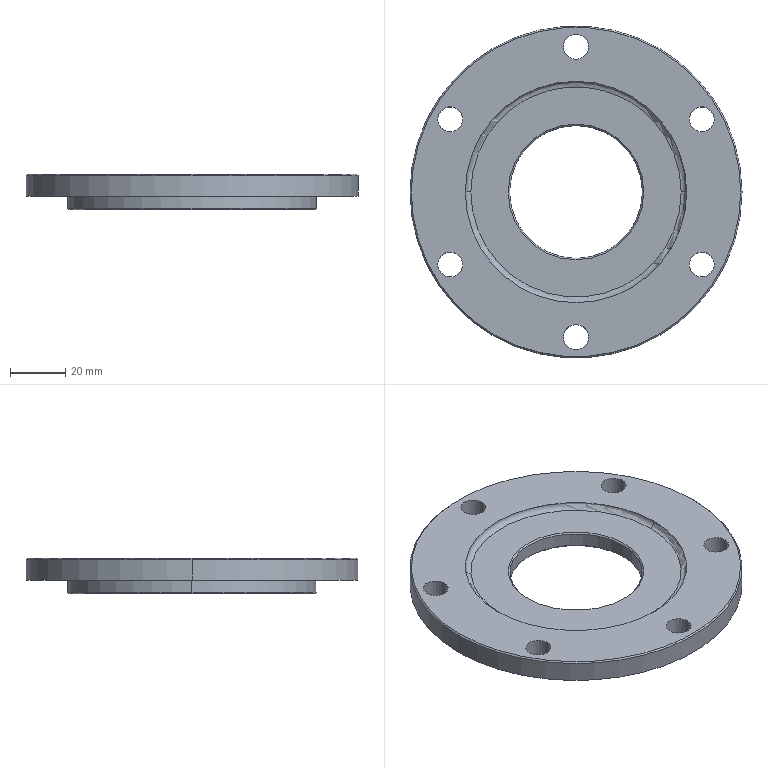Part | SolidWorks | features ICE 3, Chamfer 2, Extrusion 1, Fillet 1 | 1 solid | 35 faces | box 120 x 120 x 13 mm | volume 73283 mm3 | cylinder 20 | cone 8 | plane 5 | torus 2 | commonest cylinder face diameters 9 x12 48 x2 80 x2 90 x2 120 x2
STEP:
#1=CARTESIAN_POINT('',(-24.,0.,5.5));
#2=VERTEX_POINT('',#1);
#3=CARTESIAN_POINT('',(24.,0.,5.5));
#4=VERTEX_POINT('',#3);
#5=CARTESIAN_POINT('',(0.,0.,5.5));
#6=DIRECTION('',(0.,0.,1.));
#7=DIRECTION('',(1.,0.,0.));
#8=AXIS2_PLACEMENT_3D('',#5,#6,#7);
#9=CIRCLE('',#8,24.);
#10=EDGE_CURVE('',#2,#4,#9,.T.);
#11=ORIENTED_EDGE('',*,*,#10,.F.);
#12=CARTESIAN_POINT('',(-24.5,0.,6.));
#13=VERTEX_POINT('',#12);
#14=CARTESIAN_POINT('',(-24.,0.,5.5));
#15=DIRECTION('',(-0.7071,0.,0.7071));
#16=VECTOR('',#15,1000.);
#17=LINE('',#14,#16);
#18=EDGE_CURVE('',#2,#13,#17,.T.);
#19=ORIENTED_EDGE('',*,*,#18,.T.);
#20=CARTESIAN_POINT('',(24.5,0.,6.));
#21=VERTEX_POINT('',#20);
#22=CARTESIAN_POINT('',(0.,0.,6.));
#23=DIRECTION('',(0.,0.,-1.));
#24=DIRECTION('',(1.,0.,0.));
#25=AXIS2_PLACEMENT_3D('',#22,#23,#24);
#26=CIRCLE('',#25,24.5);
#27=EDGE_CURVE('',#21,#13,#26,.T.);
#28=ORIENTED_EDGE('',*,*,#27,.F.);
#29=CARTESIAN_POINT('',(24.,0.,5.5));
#30=DIRECTION('',(0.7071,0.,0.7071));
#31=VECTOR('',#30,1000.);
#32=LINE('',#29,#31);
#33=EDGE_CURVE('',#4,#21,#32,.T.);
#34=ORIENTED_EDGE('',*,*,#33,.F.);
#35=EDGE_LOOP('',(#11,#19,#28,#34));
#36=FACE_OUTER_BOUND('',#35,.T.);
#37=CARTESIAN_POINT('',(0.,0.,5.5));
#38=DIRECTION('',(0.,0.,1.));
#39=DIRECTION('',(1.,0.,0.));
#40=AXIS2_PLACEMENT_3D('',#37,#38,#39);
#41=CONICAL_SURFACE('',#40,24.,0.7854);
#42=ADVANCED_FACE('',(#36),#41,.F.);
#43=CARTESIAN_POINT('',(24.,0.,0.5));
#44=VERTEX_POINT('',#43);
#45=CARTESIAN_POINT('',(-24.,0.,0.5));
#46=VERTEX_POINT('',#45);
#47=CARTESIAN_POINT('',(0.,0.,0.5));
#48=DIRECTION('',(0.,0.,-1.));
#49=DIRECTION('',(1.,0.,0.));
#50=AXIS2_PLACEMENT_3D('',#47,#48,#49);
#51=CIRCLE('',#50,24.);
#52=EDGE_CURVE('',#44,#46,#51,.T.);
#53=ORIENTED_EDGE('',*,*,#52,.F.);
#54=CARTESIAN_POINT('',(24.5,0.,0.));
#55=VERTEX_POINT('',#54);
#56=CARTESIAN_POINT('',(24.5,0.,0.));
#57=DIRECTION('',(0.7071,0.,-0.7071));
#58=VECTOR('',#57,1000.);
#59=LINE('',#56,#58);
#60=EDGE_CURVE('',#44,#55,#59,.T.);
#61=ORIENTED_EDGE('',*,*,#60,.T.);
#62=CARTESIAN_POINT('',(-24.5,0.,0.));
#63=VERTEX_POINT('',#62);
#64=CARTESIAN_POINT('',(0.,0.,0.));
#65=DIRECTION('',(0.,0.,1.));
#66=DIRECTION('',(1.,0.,0.));
#67=AXIS2_PLACEMENT_3D('',#64,#65,#66);
#68=CIRCLE('',#67,24.5);
#69=EDGE_CURVE('',#63,#55,#68,.T.);
#70=ORIENTED_EDGE('',*,*,#69,.F.);
#71=CARTESIAN_POINT('',(-24.5,0.,0.));
#72=DIRECTION('',(-0.7071,0.,-0.7071));
#73=VECTOR('',#72,1000.);
#74=LINE('',#71,#73);
#75=EDGE_CURVE('',#46,#63,#74,.T.);
#76=ORIENTED_EDGE('',*,*,#75,.F.);
#77=EDGE_LOOP('',(#53,#61,#70,#76));
#78=FACE_OUTER_BOUND('',#77,.T.);
#79=CARTESIAN_POINT('',(0.,0.,0.));
#80=DIRECTION('',(0.,0.,-1.));
#81=DIRECTION('',(-1.,0.,0.));
#82=AXIS2_PLACEMENT_3D('',#79,#80,#81);
#83=CONICAL_SURFACE('',#82,24.5,0.7854);
#84=ADVANCED_FACE('',(#78),#83,.F.);
#85=ORIENTED_EDGE('',*,*,#52,.T.);
#86=CARTESIAN_POINT('',(-24.,0.,-4.));
#87=DIRECTION('',(0.,0.,1.));
#88=VECTOR('',#87,1000.);
#89=LINE('',#86,#88);
#90=EDGE_CURVE('',#46,#2,#89,.T.);
#91=ORIENTED_EDGE('',*,*,#90,.T.);
#92=ORIENTED_EDGE('',*,*,#10,.T.);
#93=CARTESIAN_POINT('',(24.,0.,-4.));
#94=DIRECTION('',(0.,0.,1.));
#95=VECTOR('',#94,1000.);
#96=LINE('',#93,#95);
#97=EDGE_CURVE('',#44,#4,#96,.T.);
#98=ORIENTED_EDGE('',*,*,#97,.F.);
#99=EDGE_LOOP('',(#85,#91,#92,#98));
#100=FACE_OUTER_BOUND('',#99,.T.);
#101=CARTESIAN_POINT('',(0.,0.,-4.));
#102=DIRECTION('',(0.,0.,1.));
#103=DIRECTION('',(1.,0.,0.));
#104=AXIS2_PLACEMENT_3D('',#101,#102,#103);
#105=CYLINDRICAL_SURFACE('',#104,24.);
#106=ADVANCED_FACE('',(#100),#105,.F.);
#107=CARTESIAN_POINT('',(-38.,0.,6.));
#108=VERTEX_POINT('',#107);
#109=CARTESIAN_POINT('',(38.,0.,6.));
#110=VERTEX_POINT('',#109);
#111=CARTESIAN_POINT('',(0.,0.,6.));
#112=DIRECTION('',(0.,0.,1.));
#113=DIRECTION('',(1.,0.,0.));
#114=AXIS2_PLACEMENT_3D('',#111,#112,#113);
#115=CIRCLE('',#114,38.);
#116=EDGE_CURVE('',#108,#110,#115,.T.);
#117=ORIENTED_EDGE('',*,*,#116,.F.);
#118=CARTESIAN_POINT('',(-40.,0.,8.));
#119=VERTEX_POINT('',#118);
#120=CARTESIAN_POINT('',(-38.,0.,8.));
#121=DIRECTION('',(0.,1.,0.));
#122=DIRECTION('',(-1.,0.,0.));
#123=AXIS2_PLACEMENT_3D('',#120,#121,#122);
#124=CIRCLE('',#123,2.);
#125=EDGE_CURVE('',#108,#119,#124,.T.);
#126=ORIENTED_EDGE('',*,*,#125,.T.);
#127=CARTESIAN_POINT('',(40.,0.,8.));
#128=VERTEX_POINT('',#127);
#129=CARTESIAN_POINT('',(0.,0.,8.));
#130=DIRECTION('',(0.,0.,1.));
#131=DIRECTION('',(1.,0.,0.));
#132=AXIS2_PLACEMENT_3D('',#129,#130,#131);
#133=CIRCLE('',#132,40.);
#134=EDGE_CURVE('',#119,#128,#133,.T.);
#135=ORIENTED_EDGE('',*,*,#134,.T.);
#136=CARTESIAN_POINT('',(38.,0.,8.));
#137=DIRECTION('',(0.,-1.,0.));
#138=DIRECTION('',(0.,0.,-1.));
#139=AXIS2_PLACEMENT_3D('',#136,#137,#138);
#140=CIRCLE('',#139,2.);
#141=EDGE_CURVE('',#110,#128,#140,.T.);
#142=ORIENTED_EDGE('',*,*,#141,.F.);
#143=EDGE_LOOP('',(#117,#126,#135,#142));
#144=FACE_OUTER_BOUND('',#143,.T.);
#145=CARTESIAN_POINT('',(0.,0.,8.));
#146=DIRECTION('',(0.,0.,1.));
#147=DIRECTION('',(1.,0.,0.));
#148=AXIS2_PLACEMENT_3D('',#145,#146,#147);
#149=TOROIDAL_SURFACE('',#148,38.,2.);
#150=ADVANCED_FACE('',(#144),#149,.F.);
#151=CARTESIAN_POINT('',(59.5,0.,8.));
#152=VERTEX_POINT('',#151);
#153=CARTESIAN_POINT('',(-59.5,0.,8.));
#154=VERTEX_POINT('',#153);
#155=CARTESIAN_POINT('',(0.,0.,8.));
#156=DIRECTION('',(0.,0.,1.));
#157=DIRECTION('',(1.,0.,0.));
#158=AXIS2_PLACEMENT_3D('',#155,#156,#157);
#159=CIRCLE('',#158,59.5);
#160=EDGE_CURVE('',#152,#154,#159,.T.);
#161=ORIENTED_EDGE('',*,*,#160,.F.);
#162=CARTESIAN_POINT('',(60.,0.,7.5));
#163=VERTEX_POINT('',#162);
#164=CARTESIAN_POINT('',(59.5,0.,8.));
#165=DIRECTION('',(0.7071,0.,-0.7071));
#166=VECTOR('',#165,1000.);
#167=LINE('',#164,#166);
#168=EDGE_CURVE('',#152,#163,#167,.T.);
#169=ORIENTED_EDGE('',*,*,#168,.T.);
#170=CARTESIAN_POINT('',(-60.,0.,7.5));
#171=VERTEX_POINT('',#170);
#172=CARTESIAN_POINT('',(0.,0.,7.5));
#173=DIRECTION('',(0.,0.,-1.));
#174=DIRECTION('',(1.,0.,0.));
#175=AXIS2_PLACEMENT_3D('',#172,#173,#174);
#176=CIRCLE('',#175,60.);
#177=EDGE_CURVE('',#171,#163,#176,.T.);
#178=ORIENTED_EDGE('',*,*,#177,.F.);
#179=CARTESIAN_POINT('',(-59.5,0.,8.));
#180=DIRECTION('',(-0.7071,0.,-0.7071));
#181=VECTOR('',#180,1000.);
#182=LINE('',#179,#181);
#183=EDGE_CURVE('',#154,#171,#182,.T.);
#184=ORIENTED_EDGE('',*,*,#183,.F.);
#185=EDGE_LOOP('',(#161,#169,#178,#184));
#186=FACE_OUTER_BOUND('',#185,.T.);
#187=CARTESIAN_POINT('',(0.,0.,8.));
#188=DIRECTION('',(0.,0.,-1.));
#189=DIRECTION('',(-1.,0.,0.));
#190=AXIS2_PLACEMENT_3D('',#187,#188,#189);
#191=CONICAL_SURFACE('',#190,59.5,0.7854);
#192=ADVANCED_FACE('',(#186),#191,.T.);
#193=CARTESIAN_POINT('',(-44.5,0.,-5.));
#194=VERTEX_POINT('',#193);
#195=CARTESIAN_POINT('',(44.5,0.,-5.));
#196=VERTEX_POINT('',#195);
#197=CARTESIAN_POINT('',(0.,0.,-5.));
#198=DIRECTION('',(0.,0.,-1.));
#199=DIRECTION('',(-1.,0.,0.));
#200=AXIS2_PLACEMENT_3D('',#197,#198,#199);
#201=CIRCLE('',#200,44.5);
#202=EDGE_CURVE('',#194,#196,#201,.T.);
#203=ORIENTED_EDGE('',*,*,#202,.F.);
#204=CARTESIAN_POINT('',(-45.,0.,-4.5));
#205=VERTEX_POINT('',#204);
#206=CARTESIAN_POINT('',(-44.5,0.,-5.));
#207=DIRECTION('',(-0.7071,0.,0.7071));
#208=VECTOR('',#207,1000.);
#209=LINE('',#206,#208);
#210=EDGE_CURVE('',#194,#205,#209,.T.);
#211=ORIENTED_EDGE('',*,*,#210,.T.);
#212=CARTESIAN_POINT('',(45.,0.,-4.5));
#213=VERTEX_POINT('',#212);
#214=CARTESIAN_POINT('',(0.,0.,-4.5));
#215=DIRECTION('',(0.,0.,1.));
#216=DIRECTION('',(-1.,0.,0.));
#217=AXIS2_PLACEMENT_3D('',#214,#215,#216);
#218=CIRCLE('',#217,45.);
#219=EDGE_CURVE('',#213,#205,#218,.T.);
#220=ORIENTED_EDGE('',*,*,#219,.F.);
#221=CARTESIAN_POINT('',(44.5,0.,-5.));
#222=DIRECTION('',(0.7071,0.,0.7071));
#223=VECTOR('',#222,1000.);
#224=LINE('',#221,#223);
#225=EDGE_CURVE('',#196,#213,#224,.T.);
#226=ORIENTED_EDGE('',*,*,#225,.F.);
#227=EDGE_LOOP('',(#203,#211,#220,#226));
#228=FACE_OUTER_BOUND('',#227,.T.);
#229=CARTESIAN_POINT('',(0.,0.,-5.));
#230=DIRECTION('',(0.,0.,1.));
#231=DIRECTION('',(1.,0.,0.));
#232=AXIS2_PLACEMENT_3D('',#229,#230,#231);
#233=CONICAL_SURFACE('',#232,44.5,0.7854);
#234=ADVANCED_FACE('',(#228),#233,.T.);
#235=CARTESIAN_POINT('',(40.,0.,-5.));
#236=VERTEX_POINT('',#235);
#237=CARTESIAN_POINT('',(-40.,0.,-5.));
#238=VERTEX_POINT('',#237);
#239=CARTESIAN_POINT('',(0.,0.,-5.));
#240=DIRECTION('',(0.,0.,-1.));
#241=DIRECTION('',(-1.,0.,0.));
#242=AXIS2_PLACEMENT_3D('',#239,#240,#241);
#243=CIRCLE('',#242,40.);
#244=EDGE_CURVE('',#236,#238,#243,.T.);
#245=ORIENTED_EDGE('',*,*,#244,.T.);
#246=CARTESIAN_POINT('',(-40.,0.,0.));
#247=VERTEX_POINT('',#246);
#248=CARTESIAN_POINT('',(-40.,0.,-5.));
#249=DIRECTION('',(0.,0.,1.));
#250=VECTOR('',#249,1000.);
#251=LINE('',#248,#250);
#252=EDGE_CURVE('',#238,#247,#251,.T.);
#253=ORIENTED_EDGE('',*,*,#252,.T.);
#254=CARTESIAN_POINT('',(40.,0.,0.));
#255=VERTEX_POINT('',#254);
#256=CARTESIAN_POINT('',(0.,0.,0.));
#257=DIRECTION('',(0.,0.,-1.));
#258=DIRECTION('',(-1.,0.,0.));
#259=AXIS2_PLACEMENT_3D('',#256,#257,#258);
#260=CIRCLE('',#259,40.);
#261=EDGE_CURVE('',#255,#247,#260,.T.);
#262=ORIENTED_EDGE('',*,*,#261,.F.);
#263=CARTESIAN_POINT('',(40.,0.,-5.));
#264=DIRECTION('',(0.,0.,1.));
#265=VECTOR('',#264,1000.);
#266=LINE('',#263,#265);
#267=EDGE_CURVE('',#236,#255,#266,.T.);
#268=ORIENTED_EDGE('',*,*,#267,.F.);
#269=EDGE_LOOP('',(#245,#253,#262,#268));
#270=FACE_OUTER_BOUND('',#269,.T.);
#271=CARTESIAN_POINT('',(0.,0.,-5.));
#272=DIRECTION('',(0.,0.,1.));
#273=DIRECTION('',(1.,0.,0.));
#274=AXIS2_PLACEMENT_3D('',#271,#272,#273);
#275=CYLINDRICAL_SURFACE('',#274,40.);
#276=ADVANCED_FACE('',(#270),#275,.F.);
#277=ORIENTED_EDGE('',*,*,#219,.T.);
#278=CARTESIAN_POINT('',(-45.,0.,0.));
#279=VERTEX_POINT('',#278);
#280=CARTESIAN_POINT('',(-45.,0.,-5.));
#281=DIRECTION('',(0.,0.,1.));
#282=VECTOR('',#281,1000.);
#283=LINE('',#280,#282);
#284=EDGE_CURVE('',#205,#279,#283,.T.);
#285=ORIENTED_EDGE('',*,*,#284,.T.);
#286=CARTESIAN_POINT('',(45.,0.,0.));
#287=VERTEX_POINT('',#286);
#288=CARTESIAN_POINT('',(0.,0.,0.));
#289=DIRECTION('',(0.,0.,-1.));
#290=DIRECTION('',(1.,0.,0.));
#291=AXIS2_PLACEMENT_3D('',#288,#289,#290);
#292=CIRCLE('',#291,45.);
#293=EDGE_CURVE('',#279,#287,#292,.T.);
#294=ORIENTED_EDGE('',*,*,#293,.T.);
#295=CARTESIAN_POINT('',(45.,0.,-5.));
#296=DIRECTION('',(0.,0.,1.));
#297=VECTOR('',#296,1000.);
#298=LINE('',#295,#297);
#299=EDGE_CURVE('',#213,#287,#298,.T.);
#300=ORIENTED_EDGE('',*,*,#299,.F.);
#301=EDGE_LOOP('',(#277,#285,#294,#300));
#302=FACE_OUTER_BOUND('',#301,.T.);
#303=CARTESIAN_POINT('',(0.,0.,-5.));
#304=DIRECTION('',(0.,0.,1.));
#305=DIRECTION('',(1.,0.,0.));
#306=AXIS2_PLACEMENT_3D('',#303,#304,#305);
#307=CYLINDRICAL_SURFACE('',#306,45.);
#308=ADVANCED_FACE('',(#302),#307,.T.);
#309=CARTESIAN_POINT('',(-49.966,26.25,8.));
#310=VERTEX_POINT('',#309);
#311=CARTESIAN_POINT('',(-40.966,26.25,8.));
#312=VERTEX_POINT('',#311);
#313=CARTESIAN_POINT('',(-45.466,26.25,8.));
#314=DIRECTION('',(0.,0.,1.));
#315=DIRECTION('',(1.,0.,0.));
#316=AXIS2_PLACEMENT_3D('',#313,#314,#315);
#317=CIRCLE('',#316,4.5);
#318=EDGE_CURVE('',#310,#312,#317,.T.);
#319=ORIENTED_EDGE('',*,*,#318,.T.);
#320=CARTESIAN_POINT('',(-40.966,26.25,0.));
#321=VERTEX_POINT('',#320);
#322=CARTESIAN_POINT('',(-40.966,26.25,8.));
#323=DIRECTION('',(0.,0.,-1.));
#324=VECTOR('',#323,1000.);
#325=LINE('',#322,#324);
#326=EDGE_CURVE('',#312,#321,#325,.T.);
#327=ORIENTED_EDGE('',*,*,#326,.T.);
#328=CARTESIAN_POINT('',(-49.966,26.25,0.));
#329=VERTEX_POINT('',#328);
#330=CARTESIAN_POINT('',(-45.466,26.25,0.));
#331=DIRECTION('',(0.,0.,1.));
#332=DIRECTION('',(1.,0.,0.));
#333=AXIS2_PLACEMENT_3D('',#330,#331,#332);
#334=CIRCLE('',#333,4.5);
#335=EDGE_CURVE('',#329,#321,#334,.T.);
#336=ORIENTED_EDGE('',*,*,#335,.F.);
#337=CARTESIAN_POINT('',(-49.966,26.25,8.));
#338=DIRECTION('',(0.,0.,-1.));
#339=VECTOR('',#338,1000.);
#340=LINE('',#337,#339);
#341=EDGE_CURVE('',#310,#329,#340,.T.);
#342=ORIENTED_EDGE('',*,*,#341,.F.);
#343=EDGE_LOOP('',(#319,#327,#336,#342));
#344=FACE_OUTER_BOUND('',#343,.T.);
#345=CARTESIAN_POINT('',(-45.466,26.25,8.));
#346=DIRECTION('',(0.,0.,-1.));
#347=DIRECTION('',(-1.,0.,0.));
#348=AXIS2_PLACEMENT_3D('',#345,#346,#347);
#349=CYLINDRICAL_SURFACE('',#348,4.5);
#350=ADVANCED_FACE('',(#344),#349,.F.);
#351=CARTESIAN_POINT('',(-49.966,-26.25,8.));
#352=VERTEX_POINT('',#351);
#353=CARTESIAN_POINT('',(-40.966,-26.25,8.));
#354=VERTEX_POINT('',#353);
#355=CARTESIAN_POINT('',(-45.466,-26.25,8.));
#356=DIRECTION('',(0.,0.,1.));
#357=DIRECTION('',(1.,0.,0.));
#358=AXIS2_PLACEMENT_3D('',#355,#356,#357);
#359=CIRCLE('',#358,4.5);
#360=EDGE_CURVE('',#352,#354,#359,.T.);
#361=ORIENTED_EDGE('',*,*,#360,.T.);
#362=CARTESIAN_POINT('',(-40.966,-26.25,0.));
#363=VERTEX_POINT('',#362);
#364=CARTESIAN_POINT('',(-40.966,-26.25,8.));
#365=DIRECTION('',(0.,0.,-1.));
#366=VECTOR('',#365,1000.);
#367=LINE('',#364,#366);
#368=EDGE_CURVE('',#354,#363,#367,.T.);
#369=ORIENTED_EDGE('',*,*,#368,.T.);
#370=CARTESIAN_POINT('',(-49.966,-26.25,0.));
#371=VERTEX_POINT('',#370);
#372=CARTESIAN_POINT('',(-45.466,-26.25,0.));
#373=DIRECTION('',(0.,0.,1.));
#374=DIRECTION('',(1.,0.,0.));
#375=AXIS2_PLACEMENT_3D('',#372,#373,#374);
#376=CIRCLE('',#375,4.5);
#377=EDGE_CURVE('',#371,#363,#376,.T.);
#378=ORIENTED_EDGE('',*,*,#377,.F.);
#379=CARTESIAN_POINT('',(-49.966,-26.25,8.));
#380=DIRECTION('',(0.,0.,-1.));
#381=VECTOR('',#380,1000.);
#382=LINE('',#379,#381);
#383=EDGE_CURVE('',#352,#371,#382,.T.);
#384=ORIENTED_EDGE('',*,*,#383,.F.);
#385=EDGE_LOOP('',(#361,#369,#378,#384));
#386=FACE_OUTER_BOUND('',#385,.T.);
#387=CARTESIAN_POINT('',(-45.466,-26.25,8.));
#388=DIRECTION('',(0.,0.,-1.));
#389=DIRECTION('',(-1.,0.,0.));
#390=AXIS2_PLACEMENT_3D('',#387,#388,#389);
#391=CYLINDRICAL_SURFACE('',#390,4.5);
#392=ADVANCED_FACE('',(#386),#391,.F.);
#393=CARTESIAN_POINT('',(-4.5,-52.5,8.));
#394=VERTEX_POINT('',#393);
#395=CARTESIAN_POINT('',(4.5,-52.5,8.));
#396=VERTEX_POINT('',#395);
#397=CARTESIAN_POINT('',(0.,-52.5,8.));
#398=DIRECTION('',(0.,0.,1.));
#399=DIRECTION('',(1.,0.,0.));
#400=AXIS2_PLACEMENT_3D('',#397,#398,#399);
#401=CIRCLE('',#400,4.5);
#402=EDGE_CURVE('',#394,#396,#401,.T.);
#403=ORIENTED_EDGE('',*,*,#402,.T.);
#404=CARTESIAN_POINT('',(4.5,-52.5,0.));
#405=VERTEX_POINT('',#404);
#406=CARTESIAN_POINT('',(4.5,-52.5,8.));
#407=DIRECTION('',(0.,0.,-1.));
#408=VECTOR('',#407,1000.);
#409=LINE('',#406,#408);
#410=EDGE_CURVE('',#396,#405,#409,.T.);
#411=ORIENTED_EDGE('',*,*,#410,.T.);
#412=CARTESIAN_POINT('',(-4.5,-52.5,0.));
#413=VERTEX_POINT('',#412);
#414=CARTESIAN_POINT('',(0.,-52.5,0.));
#415=DIRECTION('',(0.,0.,1.));
#416=DIRECTION('',(1.,0.,0.));
#417=AXIS2_PLACEMENT_3D('',#414,#415,#416);
#418=CIRCLE('',#417,4.5);
#419=EDGE_CURVE('',#413,#405,#418,.T.);
#420=ORIENTED_EDGE('',*,*,#419,.F.);
#421=CARTESIAN_POINT('',(-4.5,-52.5,8.));
#422=DIRECTION('',(0.,0.,-1.));
#423=VECTOR('',#422,1000.);
#424=LINE('',#421,#423);
#425=EDGE_CURVE('',#394,#413,#424,.T.);
#426=ORIENTED_EDGE('',*,*,#425,.F.);
#427=EDGE_LOOP('',(#403,#411,#420,#426));
#428=FACE_OUTER_BOUND('',#427,.T.);
#429=CARTESIAN_POINT('',(0.,-52.5,8.));
#430=DIRECTION('',(0.,0.,-1.));
#431=DIRECTION('',(-1.,0.,0.));
#432=AXIS2_PLACEMENT_3D('',#429,#430,#431);
#433=CYLINDRICAL_SURFACE('',#432,4.5);
#434=ADVANCED_FACE('',(#428),#433,.F.);
#435=CARTESIAN_POINT('',(40.966,-26.25,8.));
#436=VERTEX_POINT('',#435);
#437=CARTESIAN_POINT('',(49.966,-26.25,8.));
#438=VERTEX_POINT('',#437);
#439=CARTESIAN_POINT('',(45.466,-26.25,8.));
#440=DIRECTION('',(0.,0.,1.));
#441=DIRECTION('',(1.,0.,0.));
#442=AXIS2_PLACEMENT_3D('',#439,#440,#441);
#443=CIRCLE('',#442,4.5);
#444=EDGE_CURVE('',#436,#438,#443,.T.);
#445=ORIENTED_EDGE('',*,*,#444,.T.);
#446=CARTESIAN_POINT('',(49.966,-26.25,0.));
#447=VERTEX_POINT('',#446);
#448=CARTESIAN_POINT('',(49.966,-26.25,8.));
#449=DIRECTION('',(0.,0.,-1.));
#450=VECTOR('',#449,1000.);
#451=LINE('',#448,#450);
#452=EDGE_CURVE('',#438,#447,#451,.T.);
#453=ORIENTED_EDGE('',*,*,#452,.T.);
#454=CARTESIAN_POINT('',(40.966,-26.25,0.));
#455=VERTEX_POINT('',#454);
#456=CARTESIAN_POINT('',(45.466,-26.25,0.));
#457=DIRECTION('',(0.,0.,1.));
#458=DIRECTION('',(1.,0.,0.));
#459=AXIS2_PLACEMENT_3D('',#456,#457,#458);
#460=CIRCLE('',#459,4.5);
#461=EDGE_CURVE('',#455,#447,#460,.T.);
#462=ORIENTED_EDGE('',*,*,#461,.F.);
#463=CARTESIAN_POINT('',(40.966,-26.25,8.));
#464=DIRECTION('',(0.,0.,-1.));
#465=VECTOR('',#464,1000.);
#466=LINE('',#463,#465);
#467=EDGE_CURVE('',#436,#455,#466,.T.);
#468=ORIENTED_EDGE('',*,*,#467,.F.);
#469=EDGE_LOOP('',(#445,#453,#462,#468));
#470=FACE_OUTER_BOUND('',#469,.T.);
#471=CARTESIAN_POINT('',(45.466,-26.25,8.));
#472=DIRECTION('',(0.,0.,-1.));
#473=DIRECTION('',(-1.,0.,0.));
#474=AXIS2_PLACEMENT_3D('',#471,#472,#473);
#475=CYLINDRICAL_SURFACE('',#474,4.5);
#476=ADVANCED_FACE('',(#470),#475,.F.);
#477=CARTESIAN_POINT('',(40.966,26.25,8.));
#478=VERTEX_POINT('',#477);
#479=CARTESIAN_POINT('',(49.966,26.25,8.));
#480=VERTEX_POINT('',#479);
#481=CARTESIAN_POINT('',(45.466,26.25,8.));
#482=DIRECTION('',(0.,0.,1.));
#483=DIRECTION('',(1.,0.,0.));
#484=AXIS2_PLACEMENT_3D('',#481,#482,#483);
#485=CIRCLE('',#484,4.5);
#486=EDGE_CURVE('',#478,#480,#485,.T.);
#487=ORIENTED_EDGE('',*,*,#486,.T.);
#488=CARTESIAN_POINT('',(49.966,26.25,0.));
#489=VERTEX_POINT('',#488);
#490=CARTESIAN_POINT('',(49.966,26.25,8.));
#491=DIRECTION('',(0.,0.,-1.));
#492=VECTOR('',#491,1000.);
#493=LINE('',#490,#492);
#494=EDGE_CURVE('',#480,#489,#493,.T.);
#495=ORIENTED_EDGE('',*,*,#494,.T.);
#496=CARTESIAN_POINT('',(40.966,26.25,0.));
#497=VERTEX_POINT('',#496);
#498=CARTESIAN_POINT('',(45.466,26.25,0.));
#499=DIRECTION('',(0.,0.,1.));
#500=DIRECTION('',(1.,0.,0.));
#501=AXIS2_PLACEMENT_3D('',#498,#499,#500);
#502=CIRCLE('',#501,4.5);
#503=EDGE_CURVE('',#497,#489,#502,.T.);
#504=ORIENTED_EDGE('',*,*,#503,.F.);
#505=CARTESIAN_POINT('',(40.966,26.25,8.));
#506=DIRECTION('',(0.,0.,-1.));
#507=VECTOR('',#506,1000.);
#508=LINE('',#505,#507);
#509=EDGE_CURVE('',#478,#497,#508,.T.);
#510=ORIENTED_EDGE('',*,*,#509,.F.);
#511=EDGE_LOOP('',(#487,#495,#504,#510));
#512=FACE_OUTER_BOUND('',#511,.T.);
#513=CARTESIAN_POINT('',(45.466,26.25,8.));
#514=DIRECTION('',(0.,0.,-1.));
#515=DIRECTION('',(-1.,0.,0.));
#516=AXIS2_PLACEMENT_3D('',#513,#514,#515);
#517=CYLINDRICAL_SURFACE('',#516,4.5);
#518=ADVANCED_FACE('',(#512),#517,.F.);
#519=CARTESIAN_POINT('',(-4.5,52.5,8.));
#520=VERTEX_POINT('',#519);
#521=CARTESIAN_POINT('',(4.5,52.5,8.));
#522=VERTEX_POINT('',#521);
#523=CARTESIAN_POINT('',(0.,52.5,8.));
#524=DIRECTION('',(0.,0.,1.));
#525=DIRECTION('',(1.,0.,0.));
#526=AXIS2_PLACEMENT_3D('',#523,#524,#525);
#527=CIRCLE('',#526,4.5);
#528=EDGE_CURVE('',#520,#522,#527,.T.);
#529=ORIENTED_EDGE('',*,*,#528,.T.);
#530=CARTESIAN_POINT('',(4.5,52.5,0.));
#531=VERTEX_POINT('',#530);
#532=CARTESIAN_POINT('',(4.5,52.5,8.));
#533=DIRECTION('',(0.,0.,-1.));
#534=VECTOR('',#533,1000.);
#535=LINE('',#532,#534);
#536=EDGE_CURVE('',#522,#531,#535,.T.);
#537=ORIENTED_EDGE('',*,*,#536,.T.);
#538=CARTESIAN_POINT('',(-4.5,52.5,0.));
#539=VERTEX_POINT('',#538);
#540=CARTESIAN_POINT('',(0.,52.5,0.));
#541=DIRECTION('',(0.,0.,1.));
#542=DIRECTION('',(1.,0.,0.));
#543=AXIS2_PLACEMENT_3D('',#540,#541,#542);
#544=CIRCLE('',#543,4.5);
#545=EDGE_CURVE('',#539,#531,#544,.T.);
#546=ORIENTED_EDGE('',*,*,#545,.F.);
#547=CARTESIAN_POINT('',(-4.5,52.5,8.));
#548=DIRECTION('',(0.,0.,-1.));
#549=VECTOR('',#548,1000.);
#550=LINE('',#547,#549);
#551=EDGE_CURVE('',#520,#539,#550,.T.);
#552=ORIENTED_EDGE('',*,*,#551,.F.);
#553=EDGE_LOOP('',(#529,#537,#546,#552));
#554=FACE_OUTER_BOUND('',#553,.T.);
#555=CARTESIAN_POINT('',(0.,52.5,8.));
#556=DIRECTION('',(0.,0.,-1.));
#557=DIRECTION('',(-1.,0.,0.));
#558=AXIS2_PLACEMENT_3D('',#555,#556,#557);
#559=CYLINDRICAL_SURFACE('',#558,4.5);
#560=ADVANCED_FACE('',(#554),#559,.F.);
#561=ORIENTED_EDGE('',*,*,#177,.T.);
#562=CARTESIAN_POINT('',(60.,0.,0.));
#563=VERTEX_POINT('',#562);
#564=CARTESIAN_POINT('',(60.,0.,8.));
#565=DIRECTION('',(0.,0.,-1.));
#566=VECTOR('',#565,1000.);
#567=LINE('',#564,#566);
#568=EDGE_CURVE('',#163,#563,#567,.T.);
#569=ORIENTED_EDGE('',*,*,#568,.T.);
#570=CARTESIAN_POINT('',(-60.,0.,0.));
#571=VERTEX_POINT('',#570);
#572=CARTESIAN_POINT('',(0.,0.,0.));
#573=DIRECTION('',(0.,0.,1.));
#574=DIRECTION('',(1.,0.,0.));
#575=AXIS2_PLACEMENT_3D('',#572,#573,#574);
#576=CIRCLE('',#575,60.);
#577=EDGE_CURVE('',#563,#571,#576,.T.);
#578=ORIENTED_EDGE('',*,*,#577,.T.);
#579=CARTESIAN_POINT('',(-60.,0.,8.));
#580=DIRECTION('',(0.,0.,-1.));
#581=VECTOR('',#580,1000.);
#582=LINE('',#579,#581);
#583=EDGE_CURVE('',#171,#571,#582,.T.);
#584=ORIENTED_EDGE('',*,*,#583,.F.);
#585=EDGE_LOOP('',(#561,#569,#578,#584));
#586=FACE_OUTER_BOUND('',#585,.T.);
#587=CARTESIAN_POINT('',(0.,0.,8.));
#588=DIRECTION('',(0.,0.,-1.));
#589=DIRECTION('',(-1.,0.,0.));
#590=AXIS2_PLACEMENT_3D('',#587,#588,#589);
#591=CYLINDRICAL_SURFACE('',#590,60.);
#592=ADVANCED_FACE('',(#586),#591,.T.);
#593=CARTESIAN_POINT('',(0.,0.,8.));
#594=DIRECTION('',(0.,0.,1.));
#595=DIRECTION('',(1.,0.,0.));
#596=AXIS2_PLACEMENT_3D('',#593,#594,#595);
#597=CIRCLE('',#596,40.);
#598=EDGE_CURVE('',#128,#119,#597,.T.);
#599=ORIENTED_EDGE('',*,*,#598,.F.);
#600=ORIENTED_EDGE('',*,*,#134,.F.);
#601=EDGE_LOOP('',(#599,#600));
#602=FACE_BOUND('',#601,.T.);
#603=CARTESIAN_POINT('',(0.,0.,8.));
#604=DIRECTION('',(0.,0.,1.));
#605=DIRECTION('',(1.,0.,0.));
#606=AXIS2_PLACEMENT_3D('',#603,#604,#605);
#607=CIRCLE('',#606,59.5);
#608=EDGE_CURVE('',#154,#152,#607,.T.);
#609=ORIENTED_EDGE('',*,*,#608,.T.);
#610=ORIENTED_EDGE('',*,*,#160,.T.);
#611=EDGE_LOOP('',(#609,#610));
#612=FACE_OUTER_BOUND('',#611,.T.);
#613=ORIENTED_EDGE('',*,*,#360,.F.);
#614=CARTESIAN_POINT('',(-45.466,-26.25,8.));
#615=DIRECTION('',(0.,0.,1.));
#616=DIRECTION('',(1.,0.,0.));
#617=AXIS2_PLACEMENT_3D('',#614,#615,#616);
#618=CIRCLE('',#617,4.5);
#619=EDGE_CURVE('',#354,#352,#618,.T.);
#620=ORIENTED_EDGE('',*,*,#619,.F.);
#621=EDGE_LOOP('',(#613,#620));
#622=FACE_BOUND('',#621,.T.);
#623=ORIENTED_EDGE('',*,*,#444,.F.);
#624=CARTESIAN_POINT('',(45.466,-26.25,8.));
#625=DIRECTION('',(0.,0.,1.));
#626=DIRECTION('',(1.,0.,0.));
#627=AXIS2_PLACEMENT_3D('',#624,#625,#626);
#628=CIRCLE('',#627,4.5);
#629=EDGE_CURVE('',#438,#436,#628,.T.);
#630=ORIENTED_EDGE('',*,*,#629,.F.);
#631=EDGE_LOOP('',(#623,#630));
#632=FACE_BOUND('',#631,.T.);
#633=ORIENTED_EDGE('',*,*,#528,.F.);
#634=CARTESIAN_POINT('',(0.,52.5,8.));
#635=DIRECTION('',(0.,0.,1.));
#636=DIRECTION('',(1.,0.,0.));
#637=AXIS2_PLACEMENT_3D('',#634,#635,#636);
#638=CIRCLE('',#637,4.5);
#639=EDGE_CURVE('',#522,#520,#638,.T.);
#640=ORIENTED_EDGE('',*,*,#639,.F.);
#641=EDGE_LOOP('',(#633,#640));
#642=FACE_BOUND('',#641,.T.);
#643=ORIENTED_EDGE('',*,*,#486,.F.);
#644=CARTESIAN_POINT('',(45.466,26.25,8.));
#645=DIRECTION('',(0.,0.,1.));
#646=DIRECTION('',(1.,0.,0.));
#647=AXIS2_PLACEMENT_3D('',#644,#645,#646);
#648=CIRCLE('',#647,4.5);
#649=EDGE_CURVE('',#480,#478,#648,.T.);
#650=ORIENTED_EDGE('',*,*,#649,.F.);
#651=EDGE_LOOP('',(#643,#650));
#652=FACE_BOUND('',#651,.T.);
#653=ORIENTED_EDGE('',*,*,#402,.F.);
#654=CARTESIAN_POINT('',(0.,-52.5,8.));
#655=DIRECTION('',(0.,0.,1.));
#656=DIRECTION('',(1.,0.,0.));
#657=AXIS2_PLACEMENT_3D('',#654,#655,#656);
#658=CIRCLE('',#657,4.5);
#659=EDGE_CURVE('',#396,#394,#658,.T.);
#660=ORIENTED_EDGE('',*,*,#659,.F.);
#661=EDGE_LOOP('',(#653,#660));
#662=FACE_BOUND('',#661,.T.);
#663=ORIENTED_EDGE('',*,*,#318,.F.);
#664=CARTESIAN_POINT('',(-45.466,26.25,8.));
#665=DIRECTION('',(0.,0.,1.));
#666=DIRECTION('',(1.,0.,0.));
#667=AXIS2_PLACEMENT_3D('',#664,#665,#666);
#668=CIRCLE('',#667,4.5);
#669=EDGE_CURVE('',#312,#310,#668,.T.);
#670=ORIENTED_EDGE('',*,*,#669,.F.);
#671=EDGE_LOOP('',(#663,#670));
#672=FACE_BOUND('',#671,.T.);
#673=CARTESIAN_POINT('',(0.,0.,8.));
#674=DIRECTION('',(0.,0.,1.));
#675=DIRECTION('',(1.,0.,0.));
#676=AXIS2_PLACEMENT_3D('',#673,#674,#675);
#677=PLANE('',#676);
#678=ADVANCED_FACE('',(#602,#612,#622,#632,#642,#652,#662,#672),#677,.T.);
#679=CARTESIAN_POINT('',(0.,0.,0.));
#680=DIRECTION('',(0.,0.,-1.));
#681=DIRECTION('',(1.,0.,0.));
#682=AXIS2_PLACEMENT_3D('',#679,#680,#681);
#683=CIRCLE('',#682,45.);
#684=EDGE_CURVE('',#287,#279,#683,.T.);
#685=ORIENTED_EDGE('',*,*,#684,.F.);
#686=ORIENTED_EDGE('',*,*,#293,.F.);
#687=EDGE_LOOP('',(#685,#686));
#688=FACE_BOUND('',#687,.T.);
#689=CARTESIAN_POINT('',(0.,0.,0.));
#690=DIRECTION('',(0.,0.,1.));
#691=DIRECTION('',(1.,0.,0.));
#692=AXIS2_PLACEMENT_3D('',#689,#690,#691);
#693=CIRCLE('',#692,60.);
#694=EDGE_CURVE('',#571,#563,#693,.T.);
#695=ORIENTED_EDGE('',*,*,#694,.F.);
#696=ORIENTED_EDGE('',*,*,#577,.F.);
#697=EDGE_LOOP('',(#695,#696));
#698=FACE_OUTER_BOUND('',#697,.T.);
#699=ORIENTED_EDGE('',*,*,#545,.T.);
#700=CARTESIAN_POINT('',(0.,52.5,0.));
#701=DIRECTION('',(0.,0.,1.));
#702=DIRECTION('',(1.,0.,0.));
#703=AXIS2_PLACEMENT_3D('',#700,#701,#702);
#704=CIRCLE('',#703,4.5);
#705=EDGE_CURVE('',#531,#539,#704,.T.);
#706=ORIENTED_EDGE('',*,*,#705,.T.);
#707=EDGE_LOOP('',(#699,#706));
#708=FACE_BOUND('',#707,.T.);
#709=ORIENTED_EDGE('',*,*,#503,.T.);
#710=CARTESIAN_POINT('',(45.466,26.25,0.));
#711=DIRECTION('',(0.,0.,1.));
#712=DIRECTION('',(1.,0.,0.));
#713=AXIS2_PLACEMENT_3D('',#710,#711,#712);
#714=CIRCLE('',#713,4.5);
#715=EDGE_CURVE('',#489,#497,#714,.T.);
#716=ORIENTED_EDGE('',*,*,#715,.T.);
#717=EDGE_LOOP('',(#709,#716));
#718=FACE_BOUND('',#717,.T.);
#719=ORIENTED_EDGE('',*,*,#461,.T.);
#720=CARTESIAN_POINT('',(45.466,-26.25,0.));
#721=DIRECTION('',(0.,0.,1.));
#722=DIRECTION('',(1.,0.,0.));
#723=AXIS2_PLACEMENT_3D('',#720,#721,#722);
#724=CIRCLE('',#723,4.5);
#725=EDGE_CURVE('',#447,#455,#724,.T.);
#726=ORIENTED_EDGE('',*,*,#725,.T.);
#727=EDGE_LOOP('',(#719,#726));
#728=FACE_BOUND('',#727,.T.);
#729=ORIENTED_EDGE('',*,*,#419,.T.);
#730=CARTESIAN_POINT('',(0.,-52.5,0.));
#731=DIRECTION('',(0.,0.,1.));
#732=DIRECTION('',(1.,0.,0.));
#733=AXIS2_PLACEMENT_3D('',#730,#731,#732);
#734=CIRCLE('',#733,4.5);
#735=EDGE_CURVE('',#405,#413,#734,.T.);
#736=ORIENTED_EDGE('',*,*,#735,.T.);
#737=EDGE_LOOP('',(#729,#736));
#738=FACE_BOUND('',#737,.T.);
#739=ORIENTED_EDGE('',*,*,#377,.T.);
#740=CARTESIAN_POINT('',(-45.466,-26.25,0.));
#741=DIRECTION('',(0.,0.,1.));
#742=DIRECTION('',(1.,0.,0.));
#743=AXIS2_PLACEMENT_3D('',#740,#741,#742);
#744=CIRCLE('',#743,4.5);
#745=EDGE_CURVE('',#363,#371,#744,.T.);
#746=ORIENTED_EDGE('',*,*,#745,.T.);
#747=EDGE_LOOP('',(#739,#746));
#748=FACE_BOUND('',#747,.T.);
#749=ORIENTED_EDGE('',*,*,#335,.T.);
#750=CARTESIAN_POINT('',(-45.466,26.25,0.));
#751=DIRECTION('',(0.,0.,1.));
#752=DIRECTION('',(1.,0.,0.));
#753=AXIS2_PLACEMENT_3D('',#750,#751,#752);
#754=CIRCLE('',#753,4.5);
#755=EDGE_CURVE('',#321,#329,#754,.T.);
#756=ORIENTED_EDGE('',*,*,#755,.T.);
#757=EDGE_LOOP('',(#749,#756));
#758=FACE_BOUND('',#757,.T.);
#759=CARTESIAN_POINT('',(0.,0.,0.));
#760=DIRECTION('',(0.,0.,1.));
#761=DIRECTION('',(1.,0.,0.));
#762=AXIS2_PLACEMENT_3D('',#759,#760,#761);
#763=PLANE('',#762);
#764=ADVANCED_FACE('',(#688,#698,#708,#718,#728,#738,#748,#758),#763,.F.);
#765=ORIENTED_EDGE('',*,*,#568,.F.);
#766=CARTESIAN_POINT('',(0.,0.,7.5));
#767=DIRECTION('',(0.,0.,-1.));
#768=DIRECTION('',(1.,0.,0.));
#769=AXIS2_PLACEMENT_3D('',#766,#767,#768);
#770=CIRCLE('',#769,60.);
#771=EDGE_CURVE('',#163,#171,#770,.T.);
#772=ORIENTED_EDGE('',*,*,#771,.T.);
#773=ORIENTED_EDGE('',*,*,#583,.T.);
#774=ORIENTED_EDGE('',*,*,#694,.T.);
#775=EDGE_LOOP('',(#765,#772,#773,#774));
#776=FACE_OUTER_BOUND('',#775,.T.);
#777=CARTESIAN_POINT('',(0.,0.,8.));
#778=DIRECTION('',(0.,0.,-1.));
#779=DIRECTION('',(-1.,0.,0.));
#780=AXIS2_PLACEMENT_3D('',#777,#778,#779);
#781=CYLINDRICAL_SURFACE('',#780,60.);
#782=ADVANCED_FACE('',(#776),#781,.T.);
#783=ORIENTED_EDGE('',*,*,#536,.F.);
#784=ORIENTED_EDGE('',*,*,#639,.T.);
#785=ORIENTED_EDGE('',*,*,#551,.T.);
#786=ORIENTED_EDGE('',*,*,#705,.F.);
#787=EDGE_LOOP('',(#783,#784,#785,#786));
#788=FACE_OUTER_BOUND('',#787,.T.);
#789=CARTESIAN_POINT('',(0.,52.5,8.));
#790=DIRECTION('',(0.,0.,-1.));
#791=DIRECTION('',(-1.,0.,0.));
#792=AXIS2_PLACEMENT_3D('',#789,#790,#791);
#793=CYLINDRICAL_SURFACE('',#792,4.5);
#794=ADVANCED_FACE('',(#788),#793,.F.);
#795=ORIENTED_EDGE('',*,*,#494,.F.);
#796=ORIENTED_EDGE('',*,*,#649,.T.);
#797=ORIENTED_EDGE('',*,*,#509,.T.);
#798=ORIENTED_EDGE('',*,*,#715,.F.);
#799=EDGE_LOOP('',(#795,#796,#797,#798));
#800=FACE_OUTER_BOUND('',#799,.T.);
#801=CARTESIAN_POINT('',(45.466,26.25,8.));
#802=DIRECTION('',(0.,0.,-1.));
#803=DIRECTION('',(-1.,0.,0.));
#804=AXIS2_PLACEMENT_3D('',#801,#802,#803);
#805=CYLINDRICAL_SURFACE('',#804,4.5);
#806=ADVANCED_FACE('',(#800),#805,.F.);
#807=ORIENTED_EDGE('',*,*,#452,.F.);
#808=ORIENTED_EDGE('',*,*,#629,.T.);
#809=ORIENTED_EDGE('',*,*,#467,.T.);
#810=ORIENTED_EDGE('',*,*,#725,.F.);
#811=EDGE_LOOP('',(#807,#808,#809,#810));
#812=FACE_OUTER_BOUND('',#811,.T.);
#813=CARTESIAN_POINT('',(45.466,-26.25,8.));
#814=DIRECTION('',(0.,0.,-1.));
#815=DIRECTION('',(-1.,0.,0.));
#816=AXIS2_PLACEMENT_3D('',#813,#814,#815);
#817=CYLINDRICAL_SURFACE('',#816,4.5);
#818=ADVANCED_FACE('',(#812),#817,.F.);
#819=ORIENTED_EDGE('',*,*,#410,.F.);
#820=ORIENTED_EDGE('',*,*,#659,.T.);
#821=ORIENTED_EDGE('',*,*,#425,.T.);
#822=ORIENTED_EDGE('',*,*,#735,.F.);
#823=EDGE_LOOP('',(#819,#820,#821,#822));
#824=FACE_OUTER_BOUND('',#823,.T.);
#825=CARTESIAN_POINT('',(0.,-52.5,8.));
#826=DIRECTION('',(0.,0.,-1.));
#827=DIRECTION('',(-1.,0.,0.));
#828=AXIS2_PLACEMENT_3D('',#825,#826,#827);
#829=CYLINDRICAL_SURFACE('',#828,4.5);
#830=ADVANCED_FACE('',(#824),#829,.F.);
#831=ORIENTED_EDGE('',*,*,#368,.F.);
#832=ORIENTED_EDGE('',*,*,#619,.T.);
#833=ORIENTED_EDGE('',*,*,#383,.T.);
#834=ORIENTED_EDGE('',*,*,#745,.F.);
#835=EDGE_LOOP('',(#831,#832,#833,#834));
#836=FACE_OUTER_BOUND('',#835,.T.);
#837=CARTESIAN_POINT('',(-45.466,-26.25,8.));
#838=DIRECTION('',(0.,0.,-1.));
#839=DIRECTION('',(-1.,0.,0.));
#840=AXIS2_PLACEMENT_3D('',#837,#838,#839);
#841=CYLINDRICAL_SURFACE('',#840,4.5);
#842=ADVANCED_FACE('',(#836),#841,.F.);
#843=ORIENTED_EDGE('',*,*,#326,.F.);
#844=ORIENTED_EDGE('',*,*,#669,.T.);
#845=ORIENTED_EDGE('',*,*,#341,.T.);
#846=ORIENTED_EDGE('',*,*,#755,.F.);
#847=EDGE_LOOP('',(#843,#844,#845,#846));
#848=FACE_OUTER_BOUND('',#847,.T.);
#849=CARTESIAN_POINT('',(-45.466,26.25,8.));
#850=DIRECTION('',(0.,0.,-1.));
#851=DIRECTION('',(-1.,0.,0.));
#852=AXIS2_PLACEMENT_3D('',#849,#850,#851);
#853=CYLINDRICAL_SURFACE('',#852,4.5);
#854=ADVANCED_FACE('',(#848),#853,.F.);
#855=CARTESIAN_POINT('',(0.,0.,-5.));
#856=DIRECTION('',(0.,0.,-1.));
#857=DIRECTION('',(-1.,0.,0.));
#858=AXIS2_PLACEMENT_3D('',#855,#856,#857);
#859=CIRCLE('',#858,44.5);
#860=EDGE_CURVE('',#196,#194,#859,.T.);
#861=ORIENTED_EDGE('',*,*,#860,.T.);
#862=ORIENTED_EDGE('',*,*,#202,.T.);
#863=EDGE_LOOP('',(#861,#862));
#864=FACE_OUTER_BOUND('',#863,.T.);
#865=ORIENTED_EDGE('',*,*,#244,.F.);
#866=CARTESIAN_POINT('',(0.,0.,-5.));
#867=DIRECTION('',(0.,0.,-1.));
#868=DIRECTION('',(-1.,0.,0.));
#869=AXIS2_PLACEMENT_3D('',#866,#867,#868);
#870=CIRCLE('',#869,40.);
#871=EDGE_CURVE('',#238,#236,#870,.T.);
#872=ORIENTED_EDGE('',*,*,#871,.F.);
#873=EDGE_LOOP('',(#865,#872));
#874=FACE_BOUND('',#873,.T.);
#875=CARTESIAN_POINT('',(0.,0.,-5.));
#876=DIRECTION('',(0.,0.,-1.));
#877=DIRECTION('',(-1.,0.,0.));
#878=AXIS2_PLACEMENT_3D('',#875,#876,#877);
#879=PLANE('',#878);
#880=ADVANCED_FACE('',(#864,#874),#879,.T.);
#881=ORIENTED_EDGE('',*,*,#284,.F.);
#882=CARTESIAN_POINT('',(0.,0.,-4.5));
#883=DIRECTION('',(0.,0.,1.));
#884=DIRECTION('',(-1.,0.,0.));
#885=AXIS2_PLACEMENT_3D('',#882,#883,#884);
#886=CIRCLE('',#885,45.);
#887=EDGE_CURVE('',#205,#213,#886,.T.);
#888=ORIENTED_EDGE('',*,*,#887,.T.);
#889=ORIENTED_EDGE('',*,*,#299,.T.);
#890=ORIENTED_EDGE('',*,*,#684,.T.);
#891=EDGE_LOOP('',(#881,#888,#889,#890));
#892=FACE_OUTER_BOUND('',#891,.T.);
#893=CARTESIAN_POINT('',(0.,0.,-5.));
#894=DIRECTION('',(0.,0.,1.));
#895=DIRECTION('',(1.,0.,0.));
#896=AXIS2_PLACEMENT_3D('',#893,#894,#895);
#897=CYLINDRICAL_SURFACE('',#896,45.);
#898=ADVANCED_FACE('',(#892),#897,.T.);
#899=ORIENTED_EDGE('',*,*,#252,.F.);
#900=ORIENTED_EDGE('',*,*,#871,.T.);
#901=ORIENTED_EDGE('',*,*,#267,.T.);
#902=CARTESIAN_POINT('',(0.,0.,0.));
#903=DIRECTION('',(0.,0.,-1.));
#904=DIRECTION('',(-1.,0.,0.));
#905=AXIS2_PLACEMENT_3D('',#902,#903,#904);
#906=CIRCLE('',#905,40.);
#907=EDGE_CURVE('',#247,#255,#906,.T.);
#908=ORIENTED_EDGE('',*,*,#907,.F.);
#909=EDGE_LOOP('',(#899,#900,#901,#908));
#910=FACE_OUTER_BOUND('',#909,.T.);
#911=CARTESIAN_POINT('',(0.,0.,-5.));
#912=DIRECTION('',(0.,0.,1.));
#913=DIRECTION('',(1.,0.,0.));
#914=AXIS2_PLACEMENT_3D('',#911,#912,#913);
#915=CYLINDRICAL_SURFACE('',#914,40.);
#916=ADVANCED_FACE('',(#910),#915,.F.);
#917=ORIENTED_EDGE('',*,*,#69,.T.);
#918=CARTESIAN_POINT('',(0.,0.,0.));
#919=DIRECTION('',(0.,0.,1.));
#920=DIRECTION('',(1.,0.,0.));
#921=AXIS2_PLACEMENT_3D('',#918,#919,#920);
#922=CIRCLE('',#921,24.5);
#923=EDGE_CURVE('',#55,#63,#922,.T.);
#924=ORIENTED_EDGE('',*,*,#923,.T.);
#925=EDGE_LOOP('',(#917,#924));
#926=FACE_BOUND('',#925,.T.);
#927=ORIENTED_EDGE('',*,*,#261,.T.);
#928=ORIENTED_EDGE('',*,*,#907,.T.);
#929=EDGE_LOOP('',(#927,#928));
#930=FACE_OUTER_BOUND('',#929,.T.);
#931=CARTESIAN_POINT('',(0.,0.,0.));
#932=DIRECTION('',(0.,0.,1.));
#933=DIRECTION('',(1.,0.,0.));
#934=AXIS2_PLACEMENT_3D('',#931,#932,#933);
#935=PLANE('',#934);
#936=ADVANCED_FACE('',(#926,#930),#935,.F.);
#937=ORIENTED_EDGE('',*,*,#210,.F.);
#938=ORIENTED_EDGE('',*,*,#860,.F.);
#939=ORIENTED_EDGE('',*,*,#225,.T.);
#940=ORIENTED_EDGE('',*,*,#887,.F.);
#941=EDGE_LOOP('',(#937,#938,#939,#940));
#942=FACE_OUTER_BOUND('',#941,.T.);
#943=CARTESIAN_POINT('',(0.,0.,-5.));
#944=DIRECTION('',(0.,0.,1.));
#945=DIRECTION('',(1.,0.,0.));
#946=AXIS2_PLACEMENT_3D('',#943,#944,#945);
#947=CONICAL_SURFACE('',#946,44.5,0.7854);
#948=ADVANCED_FACE('',(#942),#947,.T.);
#949=ORIENTED_EDGE('',*,*,#168,.F.);
#950=ORIENTED_EDGE('',*,*,#608,.F.);
#951=ORIENTED_EDGE('',*,*,#183,.T.);
#952=ORIENTED_EDGE('',*,*,#771,.F.);
#953=EDGE_LOOP('',(#949,#950,#951,#952));
#954=FACE_OUTER_BOUND('',#953,.T.);
#955=CARTESIAN_POINT('',(0.,0.,8.));
#956=DIRECTION('',(0.,0.,-1.));
#957=DIRECTION('',(-1.,0.,0.));
#958=AXIS2_PLACEMENT_3D('',#955,#956,#957);
#959=CONICAL_SURFACE('',#958,59.5,0.7854);
#960=ADVANCED_FACE('',(#954),#959,.T.);
#961=ORIENTED_EDGE('',*,*,#27,.T.);
#962=CARTESIAN_POINT('',(0.,0.,6.));
#963=DIRECTION('',(0.,0.,-1.));
#964=DIRECTION('',(1.,0.,0.));
#965=AXIS2_PLACEMENT_3D('',#962,#963,#964);
#966=CIRCLE('',#965,24.5);
#967=EDGE_CURVE('',#13,#21,#966,.T.);
#968=ORIENTED_EDGE('',*,*,#967,.T.);
#969=EDGE_LOOP('',(#961,#968));
#970=FACE_BOUND('',#969,.T.);
#971=CARTESIAN_POINT('',(0.,0.,6.));
#972=DIRECTION('',(0.,0.,1.));
#973=DIRECTION('',(1.,0.,0.));
#974=AXIS2_PLACEMENT_3D('',#971,#972,#973);
#975=CIRCLE('',#974,38.);
#976=EDGE_CURVE('',#110,#108,#975,.T.);
#977=ORIENTED_EDGE('',*,*,#976,.T.);
#978=ORIENTED_EDGE('',*,*,#116,.T.);
#979=EDGE_LOOP('',(#977,#978));
#980=FACE_OUTER_BOUND('',#979,.T.);
#981=CARTESIAN_POINT('',(0.,0.,6.));
#982=DIRECTION('',(0.,0.,1.));
#983=DIRECTION('',(1.,0.,0.));
#984=AXIS2_PLACEMENT_3D('',#981,#982,#983);
#985=PLANE('',#984);
#986=ADVANCED_FACE('',(#970,#980),#985,.T.);
#987=ORIENTED_EDGE('',*,*,#125,.F.);
#988=ORIENTED_EDGE('',*,*,#976,.F.);
#989=ORIENTED_EDGE('',*,*,#141,.T.);
#990=ORIENTED_EDGE('',*,*,#598,.T.);
#991=EDGE_LOOP('',(#987,#988,#989,#990));
#992=FACE_OUTER_BOUND('',#991,.T.);
#993=CARTESIAN_POINT('',(0.,0.,8.));
#994=DIRECTION('',(0.,0.,1.));
#995=DIRECTION('',(1.,0.,0.));
#996=AXIS2_PLACEMENT_3D('',#993,#994,#995);
#997=TOROIDAL_SURFACE('',#996,38.,2.);
#998=ADVANCED_FACE('',(#992),#997,.F.);
#999=ORIENTED_EDGE('',*,*,#90,.F.);
#1000=CARTESIAN_POINT('',(0.,0.,0.5));
#1001=DIRECTION('',(0.,0.,-1.));
#1002=DIRECTION('',(1.,0.,0.));
#1003=AXIS2_PLACEMENT_3D('',#1000,#1001,#1002);
#1004=CIRCLE('',#1003,24.);
#1005=EDGE_CURVE('',#46,#44,#1004,.T.);
#1006=ORIENTED_EDGE('',*,*,#1005,.T.);
#1007=ORIENTED_EDGE('',*,*,#97,.T.);
#1008=CARTESIAN_POINT('',(0.,0.,5.5));
#1009=DIRECTION('',(0.,0.,1.));
#1010=DIRECTION('',(1.,0.,0.));
#1011=AXIS2_PLACEMENT_3D('',#1008,#1009,#1010);
#1012=CIRCLE('',#1011,24.);
#1013=EDGE_CURVE('',#4,#2,#1012,.T.);
#1014=ORIENTED_EDGE('',*,*,#1013,.T.);
#1015=EDGE_LOOP('',(#999,#1006,#1007,#1014));
#1016=FACE_OUTER_BOUND('',#1015,.T.);
#1017=CARTESIAN_POINT('',(0.,0.,-4.));
#1018=DIRECTION('',(0.,0.,1.));
#1019=DIRECTION('',(1.,0.,0.));
#1020=AXIS2_PLACEMENT_3D('',#1017,#1018,#1019);
#1021=CYLINDRICAL_SURFACE('',#1020,24.);
#1022=ADVANCED_FACE('',(#1016),#1021,.F.);
#1023=ORIENTED_EDGE('',*,*,#60,.F.);
#1024=ORIENTED_EDGE('',*,*,#1005,.F.);
#1025=ORIENTED_EDGE('',*,*,#75,.T.);
#1026=ORIENTED_EDGE('',*,*,#923,.F.);
#1027=EDGE_LOOP('',(#1023,#1024,#1025,#1026));
#1028=FACE_OUTER_BOUND('',#1027,.T.);
#1029=CARTESIAN_POINT('',(0.,0.,0.));
#1030=DIRECTION('',(0.,0.,-1.));
#1031=DIRECTION('',(-1.,0.,0.));
#1032=AXIS2_PLACEMENT_3D('',#1029,#1030,#1031);
#1033=CONICAL_SURFACE('',#1032,24.5,0.7854);
#1034=ADVANCED_FACE('',(#1028),#1033,.F.);
#1035=ORIENTED_EDGE('',*,*,#18,.F.);
#1036=ORIENTED_EDGE('',*,*,#1013,.F.);
#1037=ORIENTED_EDGE('',*,*,#33,.T.);
#1038=ORIENTED_EDGE('',*,*,#967,.F.);
#1039=EDGE_LOOP('',(#1035,#1036,#1037,#1038));
#1040=FACE_OUTER_BOUND('',#1039,.T.);
#1041=CARTESIAN_POINT('',(0.,0.,5.5));
#1042=DIRECTION('',(0.,0.,1.));
#1043=DIRECTION('',(1.,0.,0.));
#1044=AXIS2_PLACEMENT_3D('',#1041,#1042,#1043);
#1045=CONICAL_SURFACE('',#1044,24.,0.7854);
#1046=ADVANCED_FACE('',(#1040),#1045,.F.);
#1047=CLOSED_SHELL('',(#42,#84,#106,#150,#192,#234,#276,#308,#350,#392,#434,#476,#518,#560,#592,#678,#764,#782,#794,#806,#818,#830,#842,#854,#880,#898,#916,#936,#948,#960,#986,#998,#1022,#1034,#1046));
#1048=MANIFOLD_SOLID_BREP('',#1047);
#1049=CARTESIAN_POINT('',(0.,0.,0.));
#1050=DIRECTION('',(0.,0.,1.));
#1051=DIRECTION('',(1.,0.,0.));
#1052=AXIS2_PLACEMENT_3D('',#1049,#1050,#1051);
#1053=(LENGTH_UNIT()NAMED_UNIT(*)SI_UNIT(.MILLI.,.METRE.));
#1054=UNCERTAINTY_MEASURE_WITH_UNIT(LENGTH_MEASURE(0.00001),#1053,'','');
#1055=(NAMED_UNIT(*)PLANE_ANGLE_UNIT()SI_UNIT($,.RADIAN.));
#1056=(NAMED_UNIT(*)SI_UNIT($,.STERADIAN.)SOLID_ANGLE_UNIT());
#1057=(GEOMETRIC_REPRESENTATION_CONTEXT(3)GLOBAL_UNCERTAINTY_ASSIGNED_CONTEXT((#1054))GLOBAL_UNIT_ASSIGNED_CONTEXT((#1053,#1055,#1056))REPRESENTATION_CONTEXT('',''));
#1058=ADVANCED_BREP_SHAPE_REPRESENTATION('',(#1048,#1052),#1057);